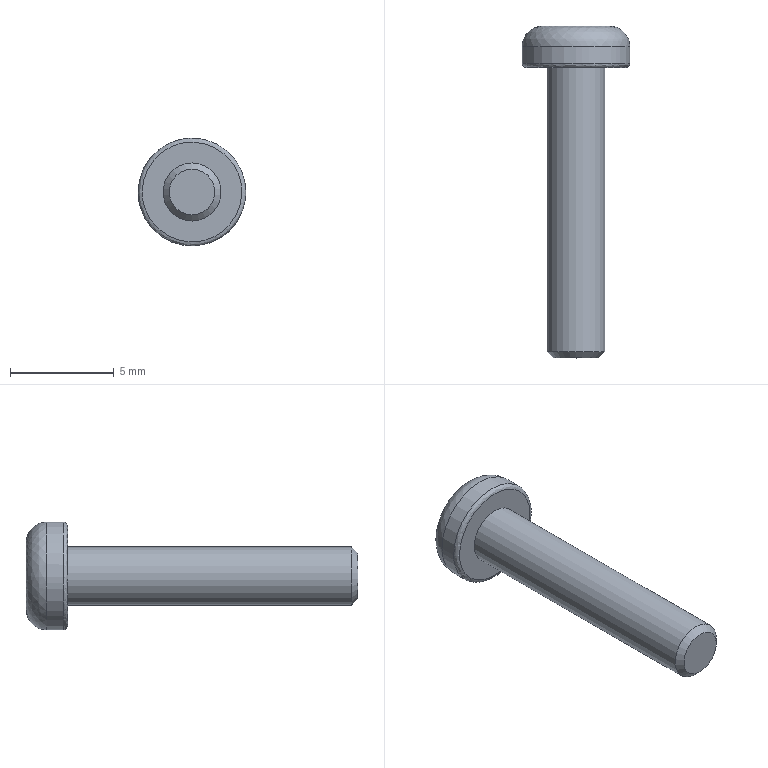Part | NX | 1 solid | 33 faces | box 5.2 x 16 x 5.2 mm | volume 120.255 mm3 | plane 16 | cylinder 14 | spline 2 | cone 1 | commonest cylinder face diameters 0.4 x6 2 x6 2.8 x1 5.2 x1